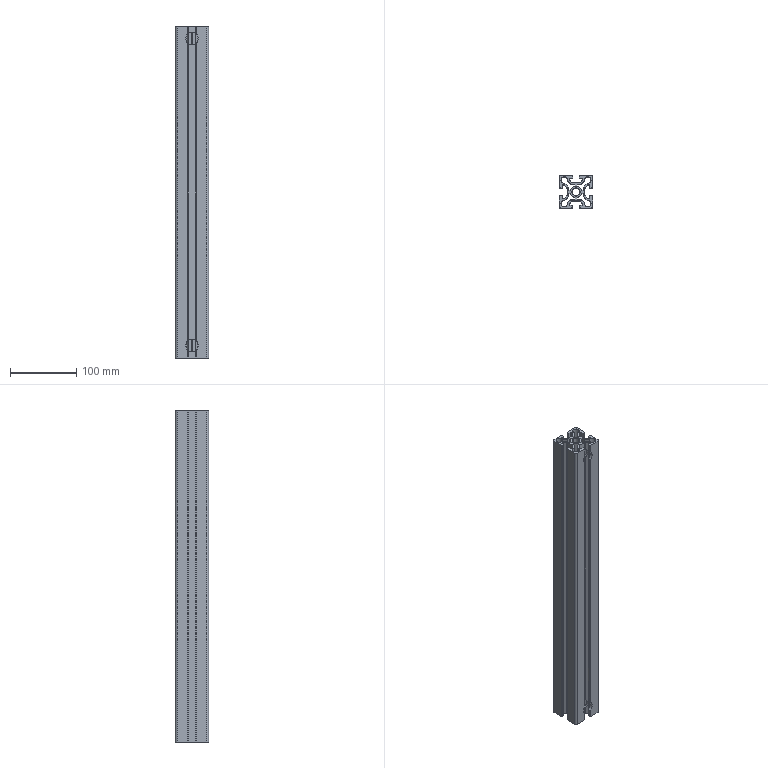Part | NX | features BREP 1 | 1 solid | 231 faces | box 50 x 50 x 500 mm | volume 489220 mm3 | plane 154 | cylinder 77 | commonest cylinder face diameters 2 x37 19 x16 10 x12 6 x4 12 x4 17 x4